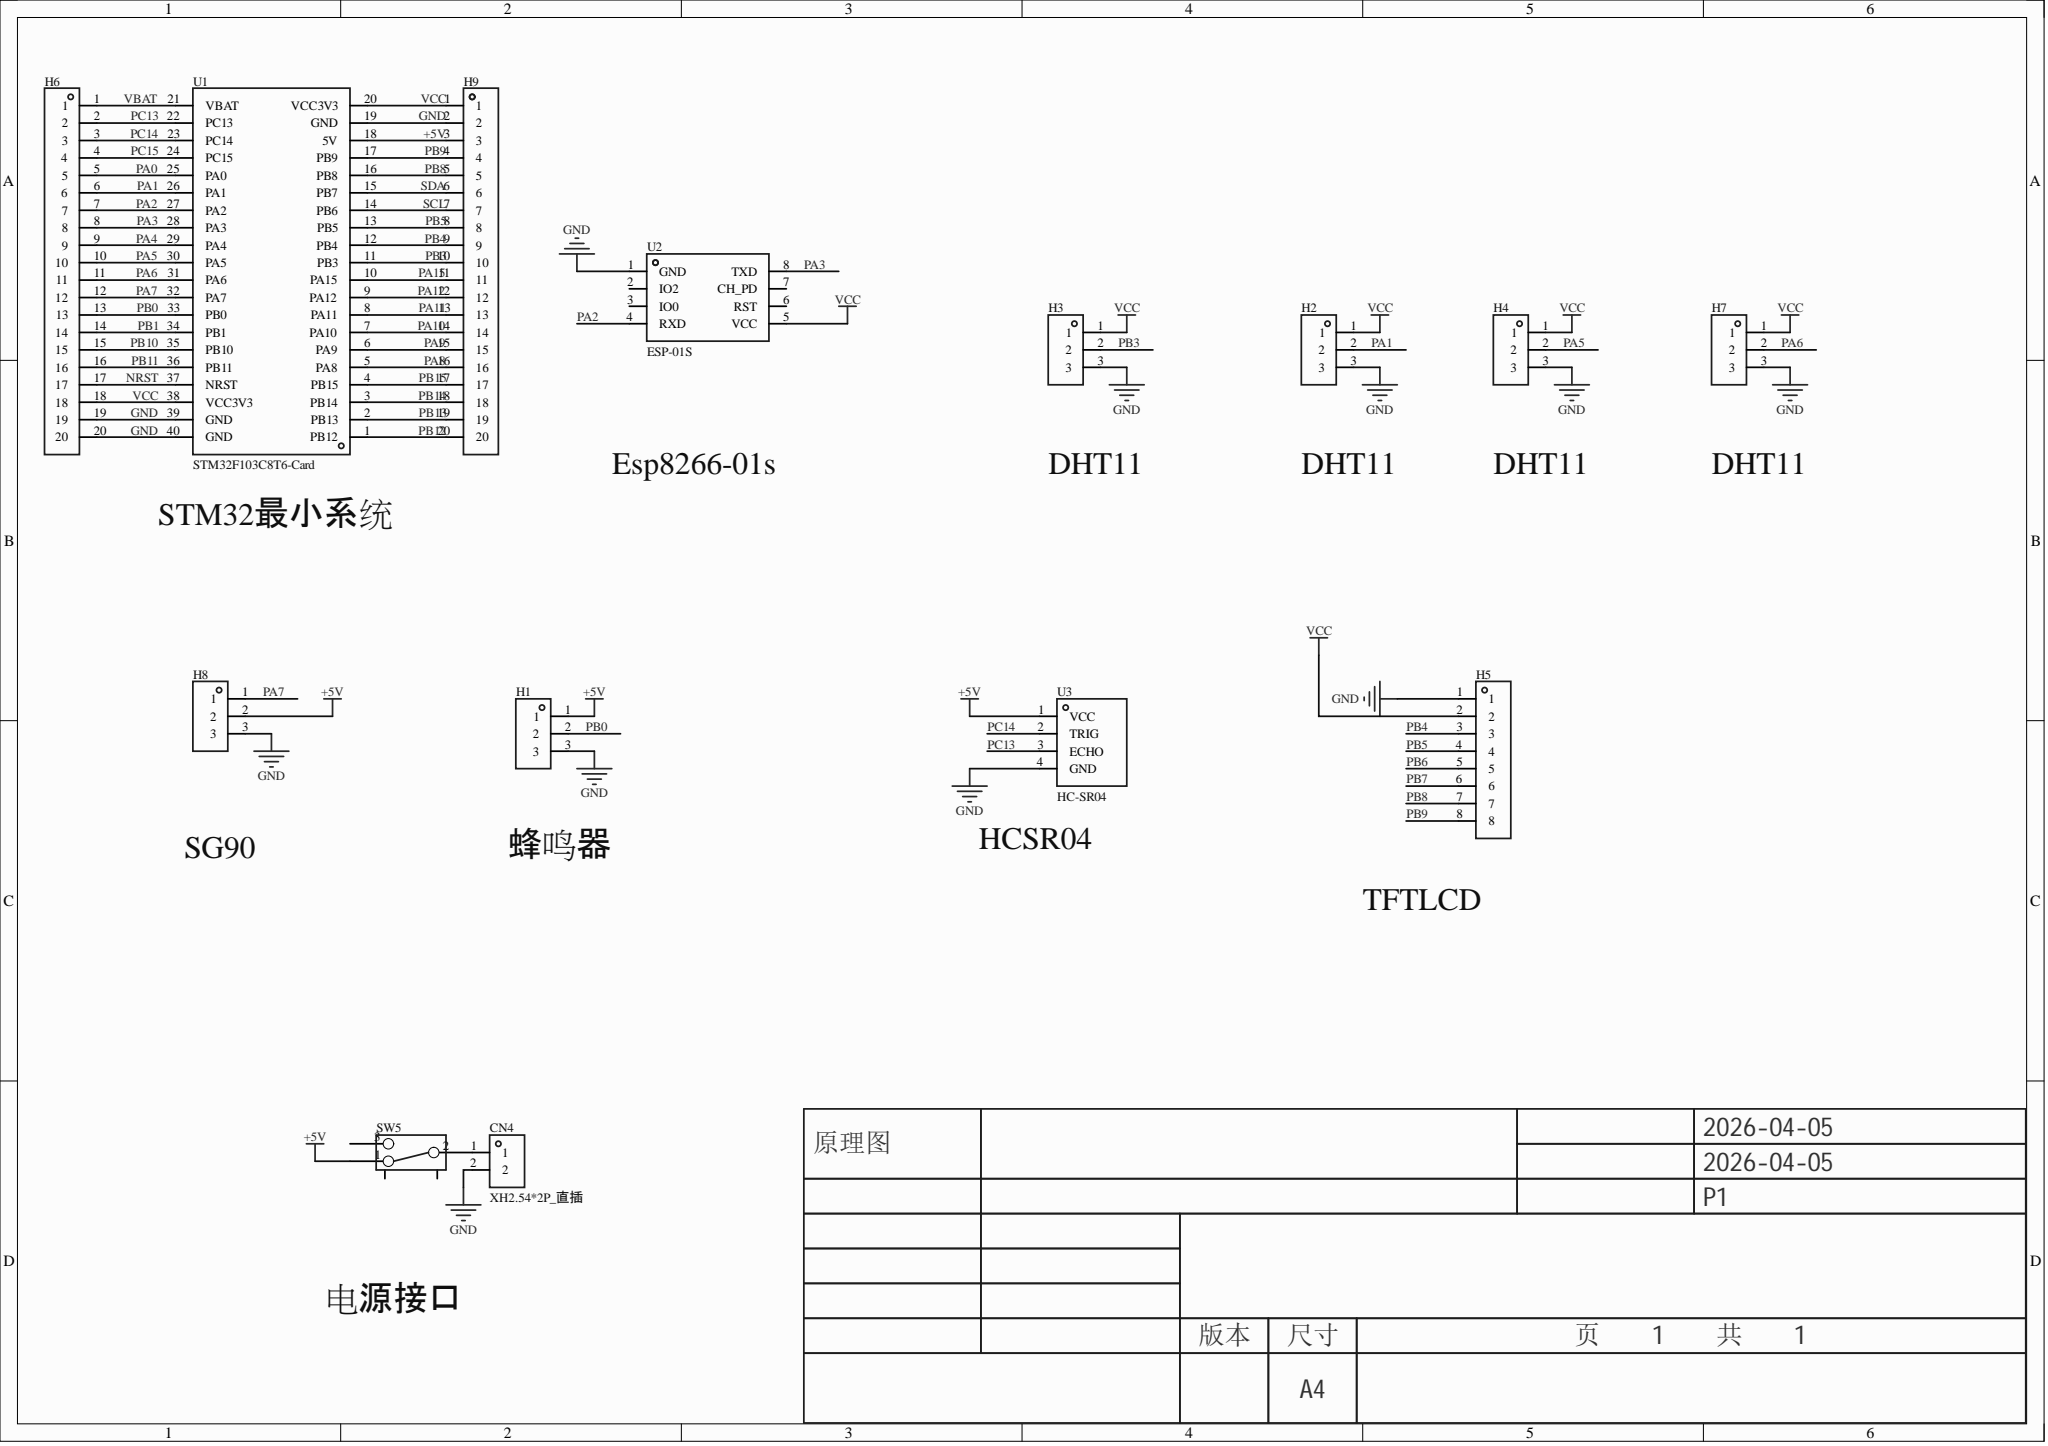Circuit board | Altium Designer | 14 parts | 38 nets
Bill of materials:
Comment,Description,Designator,Footprint,LibRef,Quantity
"XH2.54*2P_直插","","CN4","CONN-TH_2P-P2.50-XH2.54-2P","XH2.54*2P_直插","1"
"","","H1, H2, H3, H4, H7, H8","HDR-TH_3P-P2.54-V-F","HDR-F_2.54_1x3P","6"
"","","H5","HDR-TH_8P-P2.54-V-F-1","HDR-F_2.54_1x8P","1"
"","间距:2.54mm;总PIN位数:20;排数:1;插针结构:-;行距:-;安装类型:直插;圆针/方针:-;额定电流:-;额定电压:-;配合针长度:-;塑高:-;触头材质:黄铜;触头镀层:-;颜色:黑色;","H6, H9","HDR-TH_20P-P2.54-V-M-1","HDR-M_2.54_1x20P","2"
"","","SW5","拨动开关","拨动开关_正","1"
"STM32F103C8T6-Card","","U1","CONN-TH_L53.3-W22.9_STM32F103C8T6-CARD","STM32F103C8T6-Card","1"
"ESP-01S","","U2","WIFIM-TH_ESP-01S","ESP-01S_C111009","1"
"HC-SR04","","U3","TH_HC-SR04V","HC-SR04","1"
Netlist (Protel format):
[
CN4
CONN-TH_2P-P2.50-XH2.54-2P
XH2.54*2P_直插



]
[
H1
HDR-TH_3P-P2.54-V-F




]
[
H2
HDR-TH_3P-P2.54-V-F




]
[
H3
HDR-TH_3P-P2.54-V-F




]
[
H4
HDR-TH_3P-P2.54-V-F




]
[
H5
HDR-TH_8P-P2.54-V-F-1




]
[
H6
HDR-TH_20P-P2.54-V-M-1




]
[
H7
HDR-TH_3P-P2.54-V-F




]
[
H8
HDR-TH_3P-P2.54-V-F




]
[
H9
HDR-TH_20P-P2.54-V-M-1




]
[
SW5
拨动开关




]
[
U1
CONN-TH_L53.3-W22.9_STM32F103C8T6-CARD
STM32F103C8T6-Card



]
[
U2
WIFIM-TH_ESP-01S
ESP-01S



]
[
U3
TH_HC-SR04V
HC-SR04



]
(
VCC
H2-1
H3-1
H4-1
H5-2
H6-18
H7-1
H9-1
U1-20
U1-38
U2-5
)
(
VBAT
H6-1
U1-21
)
(
SDA
H9-6
U1-15
)
(
SCL
H9-7
U1-14
)
(
PC15
H6-4
U1-24
)
(
PC14
H6-3
U1-23
U3-2
)
(
PC13
H6-2
U1-22
U3-3
)
(
PB15
H9-17
U1-4
)
(
PB14
H9-18
U1-3
)
(
PB13
H9-19
U1-2
)
(
PB12
H9-20
U1-1
)
(
PB11
H6-16
U1-36
)
(
PB10
H6-15
U1-35
)
(
PB9
H5-8
H9-4
U1-17
)
(
PB8
H5-7
H9-5
U1-16
)
(
PB5
H5-4
H9-8
U1-13
)
(
PB4
H5-3
H9-9
U1-12
)
(
PB3
H3-2
H9-10
U1-11
)
(
PB1
H6-14
U1-34
)
(
PB0
H1-2
H6-13
U1-33
)
(
PA15
H9-11
U1-10
)
(
PA12
H9-12
U1-9
)
(
PA11
H9-13
U1-8
)
(
PA10
H9-14
U1-7
)
(
PA9
H9-15
U1-6
)
(
PA8
H9-16
U1-5
)
(
PA7
H6-12
H8-1
U1-32
)
(
PA6
H6-11
H7-2
U1-31
)
(
PA5
H4-2
H6-10
U1-30
)
(
PA4
H6-9
U1-29
)
(
PA3
H6-8
U1-28
U2-8
)
(
PA2
H6-7
U1-27
U2-4
)
(
PA1
H2-2
H6-6
U1-26
)
(
PA0
H6-5
U1-25
)
(
NRST
H6-17
U1-37
)
(
NetCN4_1
CN4-1
SW5-2
)
(
GND
CN4-2
H1-3
H2-3
H3-3
H4-3
H5-1
H6-19
H6-20
H7-3
H8-3
H9-2
U1-19
U1-39
U1-40
U2-1
U3-4
)
(
+5V
H1-1
H8-2
H9-3
SW5-1
U1-18
U3-1
)